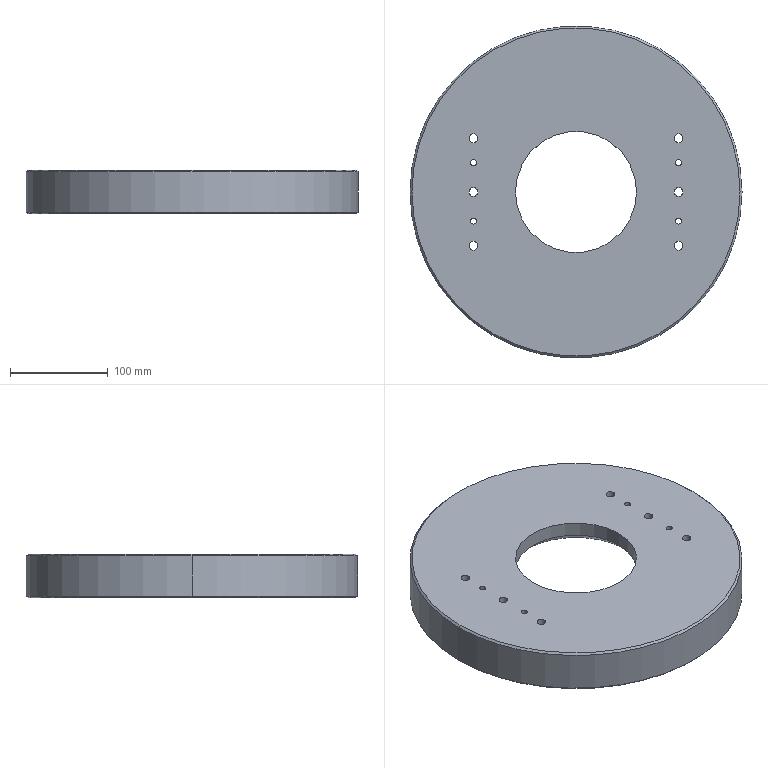NC program | NX | posted with a generic post | part box 340 x 340 x 45 mm
Lines 16251 to 17006 of 19805:
(DRILLING_COPY_1 , TOOL : D6A45)
N32488 T07 M6
N32490 G54
N32492 G17 G0 G90 X105. Y55. S3000 M3
N32494 G43 Z75. H7
N32496 G94 G81 G98 Z24. F200. R28.
N32498 Y30.
N32500 Y0.
N32502 Y-30.
N32504 Y-55.
N32506 X0. Y0.
N32508 X-105. Y55.
N32510 Y30.
N32512 Y0.
N32514 Y-30.
N32516 Y-55.
N32518 G80
N32520 G0 X-105. Y-55. Z75.
N32522 M5
(DRILLING_COPY_1_COPY_COPY_1 , TOOL : 5.8ZT)
N32524 T18 M6
N32526 G54
N32528 G17 G0 G90 X105. Y30. S2000 M3
N32530 G43 Z75. H18
N32532 G94 G83 G98 Z-3.242 F120. Q2. R28.
N32534 Y-30.
N32536 X-105.
N32538 Y30.
N32540 G80
N32542 G0 X-105. Y30. Z75.
N32544 M5
(DRILLING_COPY_1_COPY_COPY_1_COPY , TOOL : 6.0JD)
N32546 T19 M6
N32548 G54
N32550 G17 G0 G90 X105. Y30. S1000 M3
N32552 G43 Z75. H19
N32554 G94 G85 G98 Z-0.5 F40. R28.
N32556 Y-30.
N32558 X-105.
N32560 Y30.
N32562 G80
N32564 G0 X-105. Y30. Z75.
N32566 M5
(DRILLING_COPY_1_COPY_COPY_1_COPY_1 , TOOL : 9.0ZT)
N32568 T09 M6
N32570 G54
N32572 G17 G0 G90 X-105. Y55. S2000 M3
N32574 G43 Z75. H9
N32576 G94 G83 G98 Z-4.204 F120. Q2. R28.
N32578 Y0.
N32580 Y-55.
N32582 X105. Y55.
N32584 Y0.
N32586 Y-55.
N32588 G80
N32590 G0 X105. Y-55. Z75.
N32592 M5
(FLOOR_WALL_1_COPY_1 , TOOL : D10JING)
N32594 T11 M6
N32596 G54
N32598 G17 G0 G90 X0.78 Y154.4 S7000 M3
N32600 G43 Z75. H11
N32602 Z36.5
N32604 G94 G1 Z35. F1000.
N32606 G3 X-0.086 Y154.9 R1.
N32608 G1 X0.082
N32610 G2 X39.024 Y149.904 R154.9
N32612 G1 X-39.028 Y149.903
N32614 G3 X-54.739 Y144.906 R154.9
N32616 G1 X54.735 Y144.907
N32618 G2 X66.476 Y139.91 R154.9
N32620 G1 X-66.479 Y139.909
N32622 G3 X-76.11 Y134.912 R154.9
N32624 G1 X76.107 Y134.914
N32626 G2 X84.354 Y129.917 R154.9
N32628 G1 X-84.357 Y129.915
N32630 G3 X-91.594 Y124.918 R154.9
N32632 G1 X91.591 Y124.92
N32634 G2 X98.042 Y119.924 R154.9
N32636 G1 X-98.045 Y119.921
N32638 G3 X-103.857 Y114.925 R154.9
N32640 G1 X-24.462 Y114.926
N32642 X-41.497 Y109.929
N32644 X-109.132 Y109.928
N32646 G3 X-113.945 Y104.931 R154.9
N32648 G1 X-52.873 Y104.932
N32650 X-61.8 Y99.935
N32652 X-118.352 Y99.934
N32654 G3 X-122.397 Y94.937 R154.9
N32656 G1 X-69.232 Y94.938
N32658 X-75.61 Y89.941
N32660 X-126.114 Y89.94
N32662 G3 X-129.532 Y84.944 R154.9
N32664 G1 X-81.183
N32666 X-86.108 Y79.947
N32668 X-132.674
N32670 G3 X-135.56 Y74.95 R154.9
N32672 G1 X-90.491 Y74.951
N32674 X-94.407 Y69.954
N32676 X-138.205 Y69.953
N32678 G3 X-140.622 Y64.956 R154.9
N32680 G1 X-97.912 Y64.957
N32682 X-101.05 Y59.96
N32684 X-142.825
N32686 G3 X-144.821 Y54.963 R154.9
N32688 G1 X-107.5
N32690 X-105.698 Y51.395
N32692 X-106.352 Y49.967
N32694 X-146.62 Y49.966
N32696 G3 X-148.229 Y44.969 R154.9
N32698 G1 X-108.554 Y44.97
N32700 X-110.492 Y39.973
N32702 X-149.654 Y39.972
N32704 G3 X-150.9 Y34.976 R154.9
N32706 G1 X-112.174
N32708 X-113.611 Y29.979
N32710 X-151.971
N32712 G3 X-152.872 Y24.982 R154.9
N32714 G1 X-114.813 Y24.983
N32716 X-115.788 Y19.986
N32718 X-153.605 Y19.985
N32720 G3 X-154.173 Y14.989 R154.9
N32722 G1 X-116.54
N32724 X-117.074 Y9.992
N32726 X-154.577
N32728 G3 X-154.819 Y4.995 R154.9
N32730 G1 X-117.394
N32732 X-117.5 Y-0.001
N32734 X-154.9 Y-0.002
N32736 G3 X-154.819 Y-4.999 R154.9
N32738 G1 X-117.394 Y-4.998
N32740 X-117.074 Y-9.995
N32742 X-154.577
N32744 G3 X-154.173 Y-14.992 R154.9
N32746 G1 X-116.54
N32748 X-115.787 Y-19.988
N32750 X-153.605 Y-19.989
N32752 G3 X-152.872 Y-24.986 R154.9
N32754 G1 X-114.813 Y-24.985
N32756 X-113.61 Y-29.982
N32758 X-151.971
N32760 G3 X-150.899 Y-34.979 R154.9
N32762 G1 X-112.173
N32764 X-110.491 Y-39.975
N32766 X-149.653 Y-39.976
N32768 G3 X-148.228 Y-44.973 R154.9
N32770 G1 X-108.553 Y-44.972
N32772 X-106.351 Y-49.969
N32774 X-146.619
N32776 G3 X-144.82 Y-54.966 R154.9
N32778 G1 X-107.5
N32780 X-102.434 Y-57.627
N32782 X-101.048 Y-59.962
N32784 X-142.823 Y-59.963
N32786 G3 X-140.621 Y-64.96 R154.9
N32788 G1 X-97.911 Y-64.959
N32790 X-94.406 Y-69.956
N32792 X-138.203
N32794 G3 X-135.558 Y-74.953 R154.9
N32796 G1 X-90.49
N32798 X-86.107 Y-79.949
N32800 X-132.673 Y-79.95
N32802 G3 X-129.53 Y-84.947 R154.9
N32804 G1 X-81.181 Y-84.946
N32806 X-75.608 Y-89.943
N32808 X-126.112
N32810 G3 X-122.394 Y-94.94 R154.9
N32812 G1 X-69.23 Y-94.939
N32814 X-61.798 Y-99.936
N32816 X-118.35 Y-99.937
N32818 G3 X-113.943 Y-104.934 R154.9
N32820 G1 X-52.871 Y-104.933
N32822 X-41.494 Y-109.929
N32824 X-109.13 Y-109.93
N32826 G3 X-103.855 Y-114.927 R154.9
N32828 G1 X-24.459 Y-114.926
N32830 G3 X-23.593 Y-114.426 R1.
N32832 G1 Z36.5
N32834 G0 Z38.1
N32836 G1 X23.593 Y115.426 F6000.
N32838 G0 Z36.5
N32840 G1 Z35. F1000.
N32842 G3 X24.459 Y114.926 R1.
N32844 G1 X103.855 Y114.927
N32846 G2 X109.13 Y109.93 R154.9
N32848 G1 X41.494 Y109.929
N32850 X52.871 Y104.933
N32852 X113.943 Y104.934
N32854 G2 X118.35 Y99.937 R154.9
N32856 G1 X61.798 Y99.936
N32858 X69.23 Y94.939
N32860 X122.394 Y94.94
N32862 G2 X126.112 Y89.943 R154.9
N32864 G1 X75.608
N32866 X81.181 Y84.946
N32868 X129.53 Y84.947
N32870 G2 X132.673 Y79.95 R154.9
N32872 G1 X86.107 Y79.949
N32874 X90.49 Y74.953
N32876 X135.558
N32878 G2 X138.203 Y69.956 R154.9
N32880 G1 X94.406
N32882 X97.911 Y64.959
N32884 X140.621 Y64.96
N32886 G2 X142.823 Y59.963 R154.9
N32888 G1 X101.048 Y59.962
N32890 X102.434 Y57.627
N32892 X107.5 Y54.966
N32894 X144.82
N32896 G2 X146.619 Y49.969 R154.9
N32898 G1 X106.351
N32900 X108.553 Y44.972
N32902 X148.228 Y44.973
N32904 G2 X149.653 Y39.976 R154.9
N32906 G1 X110.491 Y39.975
N32908 X112.173 Y34.979
N32910 X150.899
N32912 G2 X151.971 Y29.982 R154.9
N32914 G1 X113.61
N32916 X114.813 Y24.985
N32918 X152.872 Y24.986
N32920 G2 X153.605 Y19.989 R154.9
N32922 G1 X115.787 Y19.988
N32924 X116.54 Y14.992
N32926 X154.173
N32928 G2 X154.577 Y9.995 R154.9
N32930 G1 X117.074
N32932 X117.394 Y4.998
N32934 X154.819 Y4.999
N32936 G2 X154.9 Y0.002 R154.9
N32938 G1 X117.5 Y0.001
N32940 X117.394 Y-4.995
N32942 X154.819
N32944 G2 X154.577 Y-9.992 R154.9
N32946 G1 X117.074
N32948 X116.54 Y-14.989
N32950 X154.173
N32952 G2 X153.605 Y-19.985 R154.9
N32954 G1 X115.788 Y-19.986
N32956 X114.813 Y-24.983
N32958 X152.872 Y-24.982
N32960 G2 X151.971 Y-29.979 R154.9
N32962 G1 X113.611
N32964 X112.174 Y-34.976
N32966 X150.9
N32968 G2 X149.654 Y-39.972 R154.9
N32970 G1 X110.492 Y-39.973
N32972 X108.554 Y-44.97
N32974 X148.229 Y-44.969
N32976 G2 X146.62 Y-49.966 R154.9
N32978 G1 X106.352 Y-49.967
N32980 X105.698 Y-51.395
N32982 X107.5 Y-54.963
N32984 X144.821
N32986 G2 X142.825 Y-59.96 R154.9
N32988 G1 X101.05
N32990 X97.912 Y-64.957
N32992 X140.622 Y-64.956
N32994 G2 X138.205 Y-69.953 R154.9
N32996 G1 X94.407 Y-69.954
N32998 X90.491 Y-74.951
N33000 X135.56 Y-74.95
N33002 G2 X132.674 Y-79.947 R154.9
N33004 G1 X86.108
N33006 X81.183 Y-84.944
N33008 X129.532
N33010 G2 X126.114 Y-89.94 R154.9
N33012 G1 X75.61 Y-89.941
N33014 X69.232 Y-94.938
N33016 X122.397 Y-94.937
N33018 G2 X118.352 Y-99.934 R154.9
N33020 G1 X61.8 Y-99.935
N33022 X52.873 Y-104.932
N33024 X113.945 Y-104.931
N33026 G2 X109.132 Y-109.928 R154.9
N33028 G1 X41.497 Y-109.929
N33030 X24.462 Y-114.926
N33032 X103.857 Y-114.925
N33034 G2 X98.045 Y-119.921 R154.9
N33036 G1 X-98.042 Y-119.924
N33038 G3 X-91.591 Y-124.92 R154.9
N33040 G1 X91.594 Y-124.918
N33042 G2 X84.357 Y-129.915 R154.9
N33044 G1 X-84.354 Y-129.917
N33046 G3 X-76.107 Y-134.914 R154.9
N33048 G1 X76.11 Y-134.912
N33050 G2 X66.479 Y-139.909 R154.9
N33052 G1 X-66.476 Y-139.91
N33054 G3 X-54.735 Y-144.907 R154.9
N33056 G1 X54.739 Y-144.906
N33058 G2 X39.028 Y-149.903 R154.9
N33060 G1 X-39.024 Y-149.904
N33062 G3 X-0.082 Y-154.9 R154.9
N33064 G1 X0.086
N33066 G3 X0.952 Y-154.4 R1.
N33068 G1 X-0.78 Y-154.9
N33070 G3 X0.086 Y-155.4 R1.
N33072 X155.4 Y0.086 R155.4
N33074 X0.086 Y-155.4 R-155.4
N33076 X0.952 Y-154.899 R1.
N33078 G1 X1.533 Y-153.892
N33080 Z36.5
N33082 G0 Z75.
N33084 X0.014 Y111.9
N33086 Z26.6
N33088 G1 X0.095 Z26.578
N33090 X-0.095 Z26.528
N33092 X0.095 Z26.477
N33094 X-0.095 Z26.426
N33096 X0.095 Z26.375
N33098 X-0.095 Z26.324
N33100 X0.095 Z26.273
N33102 X-0.095 Z26.222
N33104 X0.095 Z26.171
N33106 X-0.095 Z26.12
N33108 X0.095 Z26.069
N33110 X-0.095 Z26.018
N33112 X0.095 Z25.967
N33114 X-0.095 Z25.917
N33116 X0.095 Z25.866
N33118 X-0.095 Z25.815
N33120 X0.095 Z25.764
N33122 X-0.095 Z25.713
N33124 X0.095 Z25.662
N33126 X-0.095 Z25.611
N33128 X0.095 Z25.56
N33130 X-0.095 Z25.509
N33132 X0.095 Z25.458
N33134 X-0.095 Z25.407
N33136 X0.095 Z25.356
N33138 X-0.095 Z25.306
N33140 X0.095 Z25.255
N33142 X-0.095 Z25.204
N33144 X0.095 Z25.153
N33146 X-0.095 Z25.102
N33148 X0.095 Z25.051
N33150 X-0.095 Z25.
N33152 X0.095
N33154 G2 X32.989 Y106.927 R111.9
N33156 G1 X-32.99
N33158 G3 X-46.121 Y101.953 R111.9
N33160 G1 X46.121
N33162 G2 X55.825 Y96.98 R111.9
N33164 G1 X-55.826
N33166 G3 X-63.69 Y92.006 R111.9
N33168 G1 X63.689 Y92.007
N33170 G2 X70.333 Y87.034 R111.9
N33172 G1 X-70.334 Y87.033
N33174 G3 X-76.078 Y82.06 R111.9
N33176 G1 X76.077
N33178 G2 X81.112 Y77.087 R111.9
N33180 G1 X-81.113 Y77.086
N33182 G3 X-85.565 Y72.113 R111.9
N33184 G1 X85.564 Y72.114
N33186 G2 X89.52 Y67.14 R111.9
N33188 G1 X-89.52
N33190 G3 X-93.043 Y62.166 R111.9
N33192 G1 X-24.986 Y62.167
N33194 X-34.899 Y57.193
N33196 X-96.185
N33198 X-98.606 Y53.205
N33200 X-98.616 Y53.188
N33202 G2 X-99.337 Y53.067 R0.5
N33204 G1 X-102.556 Y55.524
N33206 G2 X-104.039 Y52.692 R2.5
N33208 G1 X-102.579 Y52.22
N33210 X-41.977
N33212 X-47.505 Y47.246
N33214 X-101.453
N33216 X-102.195 Y45.583
N33218 G3 X-103.608 Y42.273 R111.9
N33220 G1 X-51.981
N33222 X-55.657 Y37.3
N33224 X-105.5
N33226 G3 X-107.129 Y32.326 R111.9
N33228 G1 X-58.686
N33230 X-61.162 Y27.353
N33232 X-108.505
N33234 G3 X-109.639 Y22.38 R111.9
N33236 G1 X-63.152
N33238 X-64.699 Y17.406
N33240 X-110.538
N33242 G3 X-111.207 Y12.433 R111.9
N33244 G1 X-65.836
N33246 X-66.583 Y7.46
N33248 X-111.651
N33250 G3 X-111.872 Y2.486 R111.9
N33252 G1 X-105.261
N33254 X-105.254 Y-2.487
N33256 X-111.872
N33258 Z26.5
N33260 G0 Z28.1
N33262 G1 X-105.198 Y0.98 F6000.
N33264 G0 Z26.5
N33266 G1 Z25. F1000.
N33268 X-105.605 Y2.986
N33270 G3 X-104.739 Y2.486 R1.
N33272 G1 X-66.954
N33274 Y-2.487
N33276 X-104.746
N33278 G2 X-105.612 Y-1.987 R1.
N33280 G1 X-105.294 Y-0.956
N33282 Z26.5
N33284 G0 Z28.1
N33286 G1 X-111.651 Y-2.487 F6000.
N33288 G0 Z26.5
N33290 G1 Z25. F1000.
N33292 Y-7.46
N33294 X-66.583
N33296 X-65.836 Y-12.434
N33298 X-111.207
N33300 G3 X-110.538 Y-17.407 R111.9
N33302 G1 X-64.699
N33304 X-63.152 Y-22.38
N33306 X-109.639
N33308 G3 X-108.505 Y-27.354 R111.9
N33310 G1 X-61.162
N33312 X-58.685 Y-32.327
N33314 X-107.129
N33316 G3 X-105.5 Y-37.3 R111.9
N33318 G1 X-55.657
N33320 X-51.98 Y-42.274
N33322 X-103.608
N33324 G3 X-102.195 Y-45.583 R111.9
N33326 G1 X-101.453 Y-47.247
N33328 X-47.505
N33330 X-41.977 Y-52.22
N33332 X-97.835
N33334 X-96.185 Y-57.194
N33336 X-34.899 Y-57.193
N33338 X-24.986 Y-62.167
N33340 X-93.042
N33342 Z26.5
N33344 G0 Z28.1
N33346 G1 X23.528 Y61.128 F6000.
N33348 G0 Z26.5
N33350 G1 Z25. F1000.
N33352 X24.12 Y62.667
N33354 G3 X24.986 Y62.167 R1.
N33356 G1 X93.042
N33358 G2 X95.661 Y58.056 R111.9
N33360 G1 X96.185 Y57.194
N33362 X34.899 Y57.193
N33364 X41.977 Y52.22
N33366 X102.582
N33368 X100.186 Y51.445
N33370 G3 X99.883 Y50.766 R0.5
N33372 G1 X101.453 Y47.247
N33374 X47.505
N33376 X51.98 Y42.274
N33378 X103.608
N33380 G2 X105.5 Y37.3 R111.9
N33382 G1 X55.657
N33384 X58.685 Y32.327
N33386 X107.129
N33388 G2 X108.505 Y27.354 R111.9
N33390 G1 X61.162
N33392 X63.152 Y22.38
N33394 X109.639
N33396 G2 X110.538 Y17.407 R111.9
N33398 G1 X64.699
N33400 X65.836 Y12.434
N33402 X111.207
N33404 G2 X111.651 Y7.46 R111.9
N33406 G1 X66.583
N33408 X66.954 Y2.487
N33410 X104.746
N33412 X104.739 Y-2.486
N33414 X66.954
N33416 G2 X66.088 Y-1.986 R1.
N33418 G1 X65.493 Y-0.956
N33420 Z26.5
N33422 G0 Z28.1
N33424 G1 X104.799 Y0.98 F6000.
N33426 G0 Z26.5
N33428 G1 Z25. F1000.
N33430 X104.388 Y2.987
N33432 G3 X105.254 Y2.487 R1.
N33434 G1 X111.872
N33436 G2 X111.872 Y-2.486 R111.9
N33438 G1 X105.261
N33440 G2 X104.395 Y-1.986 R1.
N33442 G1 X104.709 Y-0.957
N33444 Z26.5
N33446 G0 Z28.1
N33448 G1 X65.216 Y-6.092 F6000.
N33450 G0 Z26.5
N33452 G1 Z25. F1000.
N33454 X65.717 Y-6.96
N33456 G3 X66.583 Y-7.46 R1.
N33458 G1 X111.651
N33460 G2 X111.207 Y-12.433 R111.9
N33462 G1 X65.836
N33464 X64.699 Y-17.406
N33466 X110.538
N33468 G2 X109.639 Y-22.38 R111.9
N33470 G1 X63.152
N33472 X61.162 Y-27.353
N33474 X108.505
N33476 G2 X107.129 Y-32.326 R111.9
N33478 G1 X58.686
N33480 X55.657 Y-37.3
N33482 X105.5
N33484 G2 X103.608 Y-42.273 R111.9
N33486 G1 X51.981
N33488 X47.505 Y-47.246
N33490 X101.453
N33492 X97.835 Y-52.22
N33494 X41.977
N33496 X34.899 Y-57.193
N33498 X96.185
N33500 X95.661 Y-58.056
N33502 G2 X93.043 Y-62.166 R111.9
N33504 G1 X24.986 Y-62.167
N33506 G2 X24.12 Y-61.667 R1.
N33508 G1 X23.758 Y-61.039
N33510 Z26.5
N33512 G0 Z28.1
N33514 G1 X-89.52 Y-62.167 F6000.
N33516 G0 Z26.5
N33518 G1 Z25. F1000.
N33520 Y-67.14
N33522 X89.52
N33524 G2 X85.565 Y-72.113 R111.9
N33526 G1 X-85.564 Y-72.114
N33528 G3 X-81.112 Y-77.087 R111.9
N33530 G1 X81.113 Y-77.086
N33532 G2 X76.078 Y-82.06 R111.9
N33534 G1 X-76.077
N33536 G3 X-70.333 Y-87.034 R111.9
N33538 G1 X70.334 Y-87.033
N33540 G2 X63.69 Y-92.006 R111.9
N33542 G1 X-63.689 Y-92.007
N33544 G3 X-55.825 Y-96.98 R111.9
N33546 G1 X55.826
N33548 G2 X46.121 Y-101.953 R111.9
N33550 G1 X-46.121
N33552 G3 X-32.989 Y-106.927 R111.9
N33554 G1 X32.99
N33556 G2 X0.095 Y-111.9 R111.9
N33558 G1 X-0.094
N33560 G2 X-0.96 Y-111.4 R1.
N33562 G1 Z26.5
N33564 G0 Z75.
N33566 X-104.504 Y-55.751
N33568 Z26.5
N33570 G1 Z25.
N33572 X-103.951 Y-56.59
N33574 G3 X-102.959 Y-56.462 R1.
N33576 G1 X-99.033 Y-53.464
N33578 X-96.089 Y-58.315
N33580 G3 X96.089 Y-58.315 R112.4
N33582 G1 X99.033 Y-53.464
N33584 X102.959 Y-56.462
N33586 G3 X103.951 Y-56.59 R1.
N33588 G1 X105.71 Y-53.233
N33590 G3 X105.04 Y-52.49 R1.
N33592 G1 X100.34 Y-50.969
N33594 X102.651 Y-45.787
N33596 G3 X102.651 Y45.787 R112.4
N33598 G1 X100.34 Y50.969
N33600 X105.04 Y52.49
N33602 G3 X105.71 Y53.233 R1.
N33604 G1 X103.951 Y56.59
N33606 G3 X102.959 Y56.462 R1.
N33608 G1 X99.033 Y53.464
N33610 X96.089 Y58.315
N33612 G3 X-96.089 Y58.315 R112.4
N33614 G1 X-99.033 Y53.464
N33616 X-102.959 Y56.462
N33618 G3 X-103.951 Y56.59 R1.
N33620 G1 X-105.71 Y53.233
N33622 G3 X-105.04 Y52.49 R1.
N33624 G1 X-100.34 Y50.969
N33626 X-102.651 Y45.787
N33628 G3 X-102.651 Y-45.787 R112.4
N33630 G1 X-100.34 Y-50.969
N33632 X-105.04 Y-52.49
N33634 G3 X-105.71 Y-53.233 R1.
N33636 G1 X-105.335 Y-54.165
N33638 Z26.5
N33640 G0 Z75.
(HOLE_MILLING , TOOL : D10JING)
N33642 X-105. Y55.
N33644 Z35.5
N33646 G3 X-106.25 Y56.25 R1.25
N33648 X-107.5 Y55. R1.25
N33650 X-107.5 Y55. Z34.5 I2.5 J0.
N33652 X-107.5 Y55. Z33.5 I2.5 J0.
N33654 X-107.5 Y55. Z32.5 I2.5 J0.
N33656 X-107.5 Y55. Z31.5 I2.5 J0.
N33658 X-107.5 Y55. Z30.5 I2.5 J0.
N33660 X-107.5 Y55. Z29.5 I2.5 J0.
N33662 X-107.5 Y55. Z28.5 I2.5 J0.
N33664 X-107.5 Y55. Z27.5 I2.5 J0.
N33666 X-107.5 Y55. Z26.5 I2.5 J0.
N33668 X-107.5 Y55. Z25.5 I2.5 J0.
N33670 X-107.5 Y55. Z24.5 I2.5 J0.
N33672 X-107.5 Y55. Z23.5 I2.5 J0.
N33674 X-107.5 Y55. Z22.5 I2.5 J0.
N33676 X-107.5 Y55. Z21.5 I2.5 J0.
N33678 X-107.5 Y55. Z20.5 I2.5 J0.
N33680 X-107.5 Y55. Z19.5 I2.5 J0.
N33682 X-107.5 Y55. Z18.5 I2.5 J0.
N33684 X-107.5 Y55. Z17.5 I2.5 J0.
N33686 X-107.5 Y55. Z16.5 I2.5 J0.
N33688 X-107.5 Y55. Z15.5 I2.5 J0.
N33690 X-102.5 Y55. Z15. I2.5 J0.
N33692 X-105. Y57.5 R2.5
N33694 X-102.5 Y55. R-2.5
N33696 X-103.75 Y56.25 R1.25
N33698 X-105. Y55. R1.25
N33700 G0 Z75.
N33702 X105.
N33704 Z35.5
N33706 G3 X103.75 Y56.25 R1.25
N33708 X102.5 Y55. R1.25
N33710 X102.5 Y55. Z34.5 I2.5 J0.
N33712 X102.5 Y55. Z33.5 I2.5 J0.
N33714 X102.5 Y55. Z32.5 I2.5 J0.
N33716 X102.5 Y55. Z31.5 I2.5 J0.
N33718 X102.5 Y55. Z30.5 I2.5 J0.
N33720 X102.5 Y55. Z29.5 I2.5 J0.
N33722 X102.5 Y55. Z28.5 I2.5 J0.
N33724 X102.5 Y55. Z27.5 I2.5 J0.
N33726 X102.5 Y55. Z26.5 I2.5 J0.
N33728 X102.5 Y55. Z25.5 I2.5 J0.
N33730 X102.5 Y55. Z24.5 I2.5 J0.
N33732 X102.5 Y55. Z23.5 I2.5 J0.
N33734 X102.5 Y55. Z22.5 I2.5 J0.
N33736 X102.5 Y55. Z21.5 I2.5 J0.
N33738 X102.5 Y55. Z20.5 I2.5 J0.
N33740 X102.5 Y55. Z19.5 I2.5 J0.
N33742 X102.5 Y55. Z18.5 I2.5 J0.
N33744 X102.5 Y55. Z17.5 I2.5 J0.
N33746 X102.5 Y55. Z16.5 I2.5 J0.
N33748 X102.5 Y55. Z15.5 I2.5 J0.
N33750 X107.5 Y55. Z15. I2.5 J0.
N33752 X105. Y57.5 R2.5
N33754 X107.5 Y55. R-2.5
N33756 X106.25 Y56.25 R1.25
N33758 X105. Y55. R1.25
N33760 G0 Z75.
N33762 Y0.
N33764 Z25.5
N33766 G3 X103.75 Y1.25 R1.25
N33768 X102.5 Y0. R1.25
N33770 X102.5 Y0. Z24.5 I2.5 J0.
N33772 X102.5 Y0. Z23.5 I2.5 J0.
N33774 X102.5 Y0. Z22.5 I2.5 J0.
N33776 X102.5 Y0. Z21.5 I2.5 J0.
N33778 X102.5 Y0. Z20.5 I2.5 J0.
N33780 X102.5 Y0. Z19.5 I2.5 J0.
N33782 X102.5 Y0. Z18.5 I2.5 J0.
N33784 X102.5 Y0. Z17.5 I2.5 J0.
N33786 X102.5 Y0. Z16.5 I2.5 J0.
N33788 X102.5 Y0. Z15.5 I2.5 J0.
N33790 X107.5 Y0. Z15. I2.5 J0.
N33792 X105. Y2.5 R2.5
N33794 X107.5 Y0. R-2.5
N33796 X106.25 Y1.25 R1.25
N33798 X105. Y0. R1.25
N33800 G0 Z75.
N33802 Y-55.
N33804 Z35.5
N33806 G3 X103.75 Y-53.75 R1.25
N33808 X102.5 Y-55. R1.25
N33810 X102.5 Y-55. Z34.5 I2.5 J0.
N33812 X102.5 Y-55. Z33.5 I2.5 J0.
N33814 X102.5 Y-55. Z32.5 I2.5 J0.
N33816 X102.5 Y-55. Z31.5 I2.5 J0.
N33818 X102.5 Y-55. Z30.5 I2.5 J0.
N33820 X102.5 Y-55. Z29.5 I2.5 J0.
N33822 X102.5 Y-55. Z28.5 I2.5 J0.
N33824 X102.5 Y-55. Z27.5 I2.5 J0.
N33826 X102.5 Y-55. Z26.5 I2.5 J0.
N33828 X102.5 Y-55. Z25.5 I2.5 J0.
N33830 X102.5 Y-55. Z24.5 I2.5 J0.
N33832 X102.5 Y-55. Z23.5 I2.5 J0.
N33834 X102.5 Y-55. Z22.5 I2.5 J0.
N33836 X102.5 Y-55. Z21.5 I2.5 J0.
N33838 X102.5 Y-55. Z20.5 I2.5 J0.
N33840 X102.5 Y-55. Z19.5 I2.5 J0.
N33842 X102.5 Y-55. Z18.5 I2.5 J0.
N33844 X102.5 Y-55. Z17.5 I2.5 J0.
N33846 X102.5 Y-55. Z16.5 I2.5 J0.
N33848 X102.5 Y-55. Z15.5 I2.5 J0.
N33850 X107.5 Y-55. Z15. I2.5 J0.
N33852 X105. Y-52.5 R2.5
N33854 X107.5 Y-55. R-2.5
N33856 X106.25 Y-53.75 R1.25
N33858 X105. Y-55. R1.25
N33860 G0 Z75.
N33862 X-105. Y0.
N33864 Z25.5
N33866 G3 X-106.25 Y1.25 R1.25
N33868 X-107.5 Y0. R1.25
N33870 X-107.5 Y0. Z24.5 I2.5 J0.
N33872 X-107.5 Y0. Z23.5 I2.5 J0.
N33874 X-107.5 Y0. Z22.5 I2.5 J0.
N33876 X-107.5 Y0. Z21.5 I2.5 J0.
N33878 X-107.5 Y0. Z20.5 I2.5 J0.
N33880 X-107.5 Y0. Z19.5 I2.5 J0.
N33882 X-107.5 Y0. Z18.5 I2.5 J0.
N33884 X-107.5 Y0. Z17.5 I2.5 J0.
N33886 X-107.5 Y0. Z16.5 I2.5 J0.
N33888 X-107.5 Y0. Z15.5 I2.5 J0.
N33890 X-102.5 Y0. Z15. I2.5 J0.
N33892 X-105. Y2.5 R2.5
N33894 X-102.5 Y0. R-2.5
N33896 X-103.75 Y1.25 R1.25
N33898 X-105. Y0. R1.25
N33900 G0 Z75.
N33902 Y-55.
N33904 Z35.5
N33906 G3 X-106.25 Y-53.75 R1.25
N33908 X-107.5 Y-55. R1.25
N33910 X-107.5 Y-55. Z34.5 I2.5 J0.
N33912 X-107.5 Y-55. Z33.5 I2.5 J0.
N33914 X-107.5 Y-55. Z32.5 I2.5 J0.
N33916 X-107.5 Y-55. Z31.5 I2.5 J0.
N33918 X-107.5 Y-55. Z30.5 I2.5 J0.
N33920 X-107.5 Y-55. Z29.5 I2.5 J0.
N33922 X-107.5 Y-55. Z28.5 I2.5 J0.
N33924 X-107.5 Y-55. Z27.5 I2.5 J0.
N33926 X-107.5 Y-55. Z26.5 I2.5 J0.
N33928 X-107.5 Y-55. Z25.5 I2.5 J0.
N33930 X-107.5 Y-55. Z24.5 I2.5 J0.
N33932 X-107.5 Y-55. Z23.5 I2.5 J0.
N33934 X-107.5 Y-55. Z22.5 I2.5 J0.
N33936 X-107.5 Y-55. Z21.5 I2.5 J0.
N33938 X-107.5 Y-55. Z20.5 I2.5 J0.
N33940 X-107.5 Y-55. Z19.5 I2.5 J0.
N33942 X-107.5 Y-55. Z18.5 I2.5 J0.
N33944 X-107.5 Y-55. Z17.5 I2.5 J0.
N33946 X-107.5 Y-55. Z16.5 I2.5 J0.
N33948 X-107.5 Y-55. Z15.5 I2.5 J0.
N33950 X-102.5 Y-55. Z15. I2.5 J0.
N33952 X-105. Y-52.5 R2.5
N33954 X-102.5 Y-55. R-2.5
N33956 X-103.75 Y-53.75 R1.25
N33958 X-105. Y-55. R1.25
N33960 G0 Z75.
N33962 M5